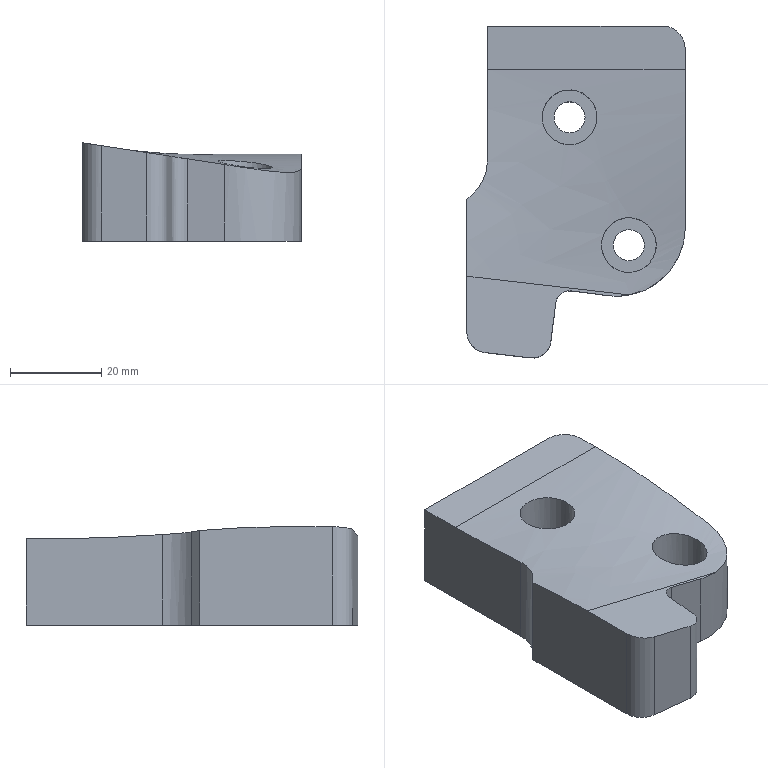Part | STEP file | gslz 2016.10.28-13_id666_x_t | 1 solid | 24 faces | box 47.84 x 72.734 x 21.542 mm | volume 50437 mm3 | plane 13 | cylinder 10 | spline 1 | commonest cylinder face diameters 6.8 x2 12 x2 6 x1 8 x1 9 x1 10 x1